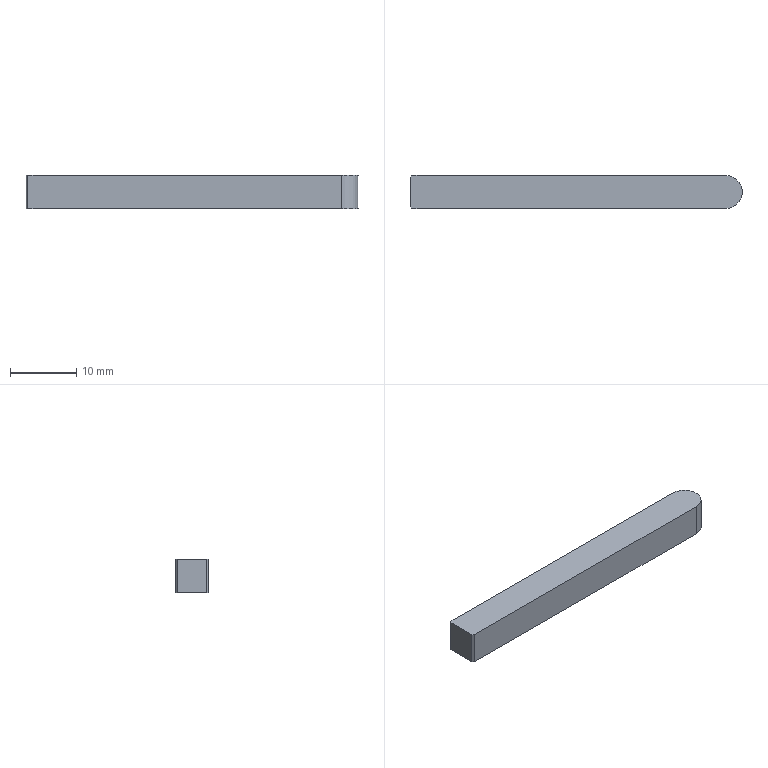Part | STEP file | BLC13-B5-L50^Magnetic powder brake assembly | 1 solid | 8 faces | box 50 x 5 x 5 mm | volume 1236 mm3 | plane 7 | cylinder 1 | commonest cylinder face diameters 5 x1
STEP:
#1=CARTESIAN_POINT('',(0.,0.,0.));
#2=DIRECTION('',(0.,0.,1.));
#3=DIRECTION('',(1.,0.,0.));
#4=AXIS2_PLACEMENT_3D('',#1,#2,#3);
#5=CARTESIAN_POINT('',(-25.,-2.2,0.));
#6=VERTEX_POINT('',#5);
#7=CARTESIAN_POINT('',(-24.7,-2.5,0.));
#8=VERTEX_POINT('',#7);
#9=CARTESIAN_POINT('',(-25.,-2.2,0.));
#10=DIRECTION('',(0.7071,-0.7071,0.));
#11=VECTOR('',#10,1.);
#12=LINE('',#9,#11);
#13=CARTESIAN_POINT('',(-25.,-2.2,5.));
#14=DIRECTION('',(0.7071,0.7071,0.));
#15=DIRECTION('',(0.,0.,-1.));
#16=AXIS2_PLACEMENT_3D('',#13,#14,#15);
#17=PLANE('',#16);
#18=CARTESIAN_POINT('',(5.,0.));
#19=DIRECTION('',(0.,-1.));
#20=VECTOR('',#19,1.);
#21=LINE('',#18,#20);
#22=(GEOMETRIC_REPRESENTATION_CONTEXT(2)PARAMETRIC_REPRESENTATION_CONTEXT()REPRESENTATION_CONTEXT('',''));
#23=DEFINITIONAL_REPRESENTATION('',(#21),#22);
#24=PCURVE('',#17,#23);
#25=CARTESIAN_POINT('',(22.5,0.,0.));
#26=DIRECTION('',(0.,0.,1.));
#27=DIRECTION('',(1.,0.,0.));
#28=AXIS2_PLACEMENT_3D('',#25,#26,#27);
#29=PLANE('',#28);
#30=CARTESIAN_POINT('',(-47.5,-2.2));
#31=DIRECTION('',(0.7071,-0.7071));
#32=VECTOR('',#31,1.);
#33=LINE('',#30,#32);
#34=(GEOMETRIC_REPRESENTATION_CONTEXT(2)PARAMETRIC_REPRESENTATION_CONTEXT()REPRESENTATION_CONTEXT('',''));
#35=DEFINITIONAL_REPRESENTATION('',(#33),#34);
#36=PCURVE('',#29,#35);
#37=SURFACE_CURVE('',#12,(#24,#36),.PCURVE_S1.);
#38=EDGE_CURVE('',#6,#8,#37,.T.);
#39=ORIENTED_EDGE('',*,*,#38,.T.);
#40=CARTESIAN_POINT('',(-24.7,-2.5,5.));
#41=VERTEX_POINT('',#40);
#42=CARTESIAN_POINT('',(-24.7,-2.5,5.));
#43=DIRECTION('',(0.,0.,-1.));
#44=VECTOR('',#43,1.);
#45=LINE('',#42,#44);
#46=CARTESIAN_POINT('',(0.,-0.4243));
#47=DIRECTION('',(1.,0.));
#48=VECTOR('',#47,1.);
#49=LINE('',#46,#48);
#50=(GEOMETRIC_REPRESENTATION_CONTEXT(2)PARAMETRIC_REPRESENTATION_CONTEXT()REPRESENTATION_CONTEXT('',''));
#51=DEFINITIONAL_REPRESENTATION('',(#49),#50);
#52=PCURVE('',#17,#51);
#53=CARTESIAN_POINT('',(-24.7,-2.5,5.));
#54=DIRECTION('',(0.,1.,0.));
#55=DIRECTION('',(1.,0.,0.));
#56=AXIS2_PLACEMENT_3D('',#53,#54,#55);
#57=PLANE('',#56);
#58=CARTESIAN_POINT('',(0.,0.));
#59=DIRECTION('',(0.,1.));
#60=VECTOR('',#59,1.);
#61=LINE('',#58,#60);
#62=(GEOMETRIC_REPRESENTATION_CONTEXT(2)PARAMETRIC_REPRESENTATION_CONTEXT()REPRESENTATION_CONTEXT('',''));
#63=DEFINITIONAL_REPRESENTATION('',(#61),#62);
#64=PCURVE('',#57,#63);
#65=SURFACE_CURVE('',#45,(#52,#64),.PCURVE_S1.);
#66=EDGE_CURVE('',#41,#8,#65,.T.);
#67=ORIENTED_EDGE('',*,*,#66,.F.);
#68=CARTESIAN_POINT('',(-25.,-2.2,5.));
#69=VERTEX_POINT('',#68);
#70=CARTESIAN_POINT('',(-25.,-2.2,5.));
#71=DIRECTION('',(0.7071,-0.7071,0.));
#72=VECTOR('',#71,1.);
#73=LINE('',#70,#72);
#74=CARTESIAN_POINT('',(0.,0.));
#75=DIRECTION('',(0.,-1.));
#76=VECTOR('',#75,1.);
#77=LINE('',#74,#76);
#78=(GEOMETRIC_REPRESENTATION_CONTEXT(2)PARAMETRIC_REPRESENTATION_CONTEXT()REPRESENTATION_CONTEXT('',''));
#79=DEFINITIONAL_REPRESENTATION('',(#77),#78);
#80=PCURVE('',#17,#79);
#81=CARTESIAN_POINT('',(22.5,0.,5.));
#82=DIRECTION('',(0.,0.,1.));
#83=DIRECTION('',(1.,0.,0.));
#84=AXIS2_PLACEMENT_3D('',#81,#82,#83);
#85=PLANE('',#84);
#86=CARTESIAN_POINT('',(-47.5,-2.2));
#87=DIRECTION('',(0.7071,-0.7071));
#88=VECTOR('',#87,1.);
#89=LINE('',#86,#88);
#90=(GEOMETRIC_REPRESENTATION_CONTEXT(2)PARAMETRIC_REPRESENTATION_CONTEXT()REPRESENTATION_CONTEXT('',''));
#91=DEFINITIONAL_REPRESENTATION('',(#89),#90);
#92=PCURVE('',#85,#91);
#93=SURFACE_CURVE('',#73,(#80,#92),.PCURVE_S1.);
#94=EDGE_CURVE('',#69,#41,#93,.T.);
#95=ORIENTED_EDGE('',*,*,#94,.F.);
#96=CARTESIAN_POINT('',(-25.,-2.2,5.));
#97=DIRECTION('',(0.,0.,-1.));
#98=VECTOR('',#97,1.);
#99=LINE('',#96,#98);
#100=CARTESIAN_POINT('',(0.,0.));
#101=DIRECTION('',(1.,0.));
#102=VECTOR('',#101,1.);
#103=LINE('',#100,#102);
#104=(GEOMETRIC_REPRESENTATION_CONTEXT(2)PARAMETRIC_REPRESENTATION_CONTEXT()REPRESENTATION_CONTEXT('',''));
#105=DEFINITIONAL_REPRESENTATION('',(#103),#104);
#106=PCURVE('',#17,#105);
#107=CARTESIAN_POINT('',(-25.,2.2,5.));
#108=DIRECTION('',(1.,0.,0.));
#109=DIRECTION('',(0.,1.,0.));
#110=AXIS2_PLACEMENT_3D('',#107,#108,#109);
#111=PLANE('',#110);
#112=CARTESIAN_POINT('',(-4.4,0.));
#113=DIRECTION('',(0.,-1.));
#114=VECTOR('',#113,1.);
#115=LINE('',#112,#114);
#116=(GEOMETRIC_REPRESENTATION_CONTEXT(2)PARAMETRIC_REPRESENTATION_CONTEXT()REPRESENTATION_CONTEXT('',''));
#117=DEFINITIONAL_REPRESENTATION('',(#115),#116);
#118=PCURVE('',#111,#117);
#119=SURFACE_CURVE('',#99,(#106,#118),.PCURVE_S1.);
#120=EDGE_CURVE('',#69,#6,#119,.T.);
#121=ORIENTED_EDGE('',*,*,#120,.T.);
#122=EDGE_LOOP('',(#39,#67,#95,#121));
#123=FACE_BOUND('',#122,.T.);
#124=ADVANCED_FACE('',(#123),#17,.F.);
#125=CARTESIAN_POINT('',(-24.7,2.5,0.));
#126=VERTEX_POINT('',#125);
#127=CARTESIAN_POINT('',(-25.,2.2,0.));
#128=VERTEX_POINT('',#127);
#129=CARTESIAN_POINT('',(-24.7,2.5,0.));
#130=DIRECTION('',(-0.7071,-0.7071,0.));
#131=VECTOR('',#130,1.);
#132=LINE('',#129,#131);
#133=CARTESIAN_POINT('',(-24.7,2.5,5.));
#134=DIRECTION('',(0.7071,-0.7071,0.));
#135=DIRECTION('',(0.,0.,-1.));
#136=AXIS2_PLACEMENT_3D('',#133,#134,#135);
#137=PLANE('',#136);
#138=CARTESIAN_POINT('',(5.,0.));
#139=DIRECTION('',(0.,-1.));
#140=VECTOR('',#139,1.);
#141=LINE('',#138,#140);
#142=(GEOMETRIC_REPRESENTATION_CONTEXT(2)PARAMETRIC_REPRESENTATION_CONTEXT()REPRESENTATION_CONTEXT('',''));
#143=DEFINITIONAL_REPRESENTATION('',(#141),#142);
#144=PCURVE('',#137,#143);
#145=CARTESIAN_POINT('',(-47.2,2.5));
#146=DIRECTION('',(-0.7071,-0.7071));
#147=VECTOR('',#146,1.);
#148=LINE('',#145,#147);
#149=(GEOMETRIC_REPRESENTATION_CONTEXT(2)PARAMETRIC_REPRESENTATION_CONTEXT()REPRESENTATION_CONTEXT('',''));
#150=DEFINITIONAL_REPRESENTATION('',(#148),#149);
#151=PCURVE('',#29,#150);
#152=SURFACE_CURVE('',#132,(#144,#151),.PCURVE_S1.);
#153=EDGE_CURVE('',#126,#128,#152,.T.);
#154=ORIENTED_EDGE('',*,*,#153,.T.);
#155=CARTESIAN_POINT('',(-25.,2.2,5.));
#156=VERTEX_POINT('',#155);
#157=CARTESIAN_POINT('',(-25.,2.2,5.));
#158=DIRECTION('',(0.,0.,-1.));
#159=VECTOR('',#158,1.);
#160=LINE('',#157,#159);
#161=CARTESIAN_POINT('',(0.,-0.4243));
#162=DIRECTION('',(1.,0.));
#163=VECTOR('',#162,1.);
#164=LINE('',#161,#163);
#165=(GEOMETRIC_REPRESENTATION_CONTEXT(2)PARAMETRIC_REPRESENTATION_CONTEXT()REPRESENTATION_CONTEXT('',''));
#166=DEFINITIONAL_REPRESENTATION('',(#164),#165);
#167=PCURVE('',#137,#166);
#168=CARTESIAN_POINT('',(0.,0.));
#169=DIRECTION('',(0.,-1.));
#170=VECTOR('',#169,1.);
#171=LINE('',#168,#170);
#172=(GEOMETRIC_REPRESENTATION_CONTEXT(2)PARAMETRIC_REPRESENTATION_CONTEXT()REPRESENTATION_CONTEXT('',''));
#173=DEFINITIONAL_REPRESENTATION('',(#171),#172);
#174=PCURVE('',#111,#173);
#175=SURFACE_CURVE('',#160,(#167,#174),.PCURVE_S1.);
#176=EDGE_CURVE('',#156,#128,#175,.T.);
#177=ORIENTED_EDGE('',*,*,#176,.F.);
#178=CARTESIAN_POINT('',(-24.7,2.5,5.));
#179=VERTEX_POINT('',#178);
#180=CARTESIAN_POINT('',(-24.7,2.5,5.));
#181=DIRECTION('',(-0.7071,-0.7071,0.));
#182=VECTOR('',#181,1.);
#183=LINE('',#180,#182);
#184=CARTESIAN_POINT('',(0.,0.));
#185=DIRECTION('',(0.,-1.));
#186=VECTOR('',#185,1.);
#187=LINE('',#184,#186);
#188=(GEOMETRIC_REPRESENTATION_CONTEXT(2)PARAMETRIC_REPRESENTATION_CONTEXT()REPRESENTATION_CONTEXT('',''));
#189=DEFINITIONAL_REPRESENTATION('',(#187),#188);
#190=PCURVE('',#137,#189);
#191=CARTESIAN_POINT('',(-47.2,2.5));
#192=DIRECTION('',(-0.7071,-0.7071));
#193=VECTOR('',#192,1.);
#194=LINE('',#191,#193);
#195=(GEOMETRIC_REPRESENTATION_CONTEXT(2)PARAMETRIC_REPRESENTATION_CONTEXT()REPRESENTATION_CONTEXT('',''));
#196=DEFINITIONAL_REPRESENTATION('',(#194),#195);
#197=PCURVE('',#85,#196);
#198=SURFACE_CURVE('',#183,(#190,#197),.PCURVE_S1.);
#199=EDGE_CURVE('',#179,#156,#198,.T.);
#200=ORIENTED_EDGE('',*,*,#199,.F.);
#201=CARTESIAN_POINT('',(-24.7,2.5,5.));
#202=DIRECTION('',(0.,0.,-1.));
#203=VECTOR('',#202,1.);
#204=LINE('',#201,#203);
#205=CARTESIAN_POINT('',(0.,0.));
#206=DIRECTION('',(1.,0.));
#207=VECTOR('',#206,1.);
#208=LINE('',#205,#207);
#209=(GEOMETRIC_REPRESENTATION_CONTEXT(2)PARAMETRIC_REPRESENTATION_CONTEXT()REPRESENTATION_CONTEXT('',''));
#210=DEFINITIONAL_REPRESENTATION('',(#208),#209);
#211=PCURVE('',#137,#210);
#212=CARTESIAN_POINT('',(22.5,2.5,5.));
#213=DIRECTION('',(0.,-1.,0.));
#214=DIRECTION('',(0.,0.,-1.));
#215=AXIS2_PLACEMENT_3D('',#212,#213,#214);
#216=PLANE('',#215);
#217=CARTESIAN_POINT('',(0.,-47.2));
#218=DIRECTION('',(1.,0.));
#219=VECTOR('',#218,1.);
#220=LINE('',#217,#219);
#221=(GEOMETRIC_REPRESENTATION_CONTEXT(2)PARAMETRIC_REPRESENTATION_CONTEXT()REPRESENTATION_CONTEXT('',''));
#222=DEFINITIONAL_REPRESENTATION('',(#220),#221);
#223=PCURVE('',#216,#222);
#224=SURFACE_CURVE('',#204,(#211,#223),.PCURVE_S1.);
#225=EDGE_CURVE('',#179,#126,#224,.T.);
#226=ORIENTED_EDGE('',*,*,#225,.T.);
#227=EDGE_LOOP('',(#154,#177,#200,#226));
#228=FACE_BOUND('',#227,.T.);
#229=ADVANCED_FACE('',(#228),#137,.F.);
#230=CARTESIAN_POINT('',(-25.,2.2,0.));
#231=DIRECTION('',(0.,-1.,0.));
#232=VECTOR('',#231,1.);
#233=LINE('',#230,#232);
#234=CARTESIAN_POINT('',(-47.5,2.2));
#235=DIRECTION('',(0.,-1.));
#236=VECTOR('',#235,1.);
#237=LINE('',#234,#236);
#238=(GEOMETRIC_REPRESENTATION_CONTEXT(2)PARAMETRIC_REPRESENTATION_CONTEXT()REPRESENTATION_CONTEXT('',''));
#239=DEFINITIONAL_REPRESENTATION('',(#237),#238);
#240=PCURVE('',#29,#239);
#241=CARTESIAN_POINT('',(0.,-5.));
#242=DIRECTION('',(-1.,0.));
#243=VECTOR('',#242,1.);
#244=LINE('',#241,#243);
#245=(GEOMETRIC_REPRESENTATION_CONTEXT(2)PARAMETRIC_REPRESENTATION_CONTEXT()REPRESENTATION_CONTEXT('',''));
#246=DEFINITIONAL_REPRESENTATION('',(#244),#245);
#247=PCURVE('',#111,#246);
#248=SURFACE_CURVE('',#233,(#240,#247),.PCURVE_S1.);
#249=EDGE_CURVE('',#128,#6,#248,.T.);
#250=ORIENTED_EDGE('',*,*,#249,.F.);
#251=ORIENTED_EDGE('',*,*,#153,.F.);
#252=CARTESIAN_POINT('',(22.5,2.5,0.));
#253=VERTEX_POINT('',#252);
#254=CARTESIAN_POINT('',(22.5,2.5,0.));
#255=DIRECTION('',(-1.,0.,0.));
#256=VECTOR('',#255,1.);
#257=LINE('',#254,#256);
#258=CARTESIAN_POINT('',(0.,2.5));
#259=DIRECTION('',(-1.,0.));
#260=VECTOR('',#259,1.);
#261=LINE('',#258,#260);
#262=(GEOMETRIC_REPRESENTATION_CONTEXT(2)PARAMETRIC_REPRESENTATION_CONTEXT()REPRESENTATION_CONTEXT('',''));
#263=DEFINITIONAL_REPRESENTATION('',(#261),#262);
#264=PCURVE('',#29,#263);
#265=CARTESIAN_POINT('',(5.,0.));
#266=DIRECTION('',(0.,-1.));
#267=VECTOR('',#266,1.);
#268=LINE('',#265,#267);
#269=(GEOMETRIC_REPRESENTATION_CONTEXT(2)PARAMETRIC_REPRESENTATION_CONTEXT()REPRESENTATION_CONTEXT('',''));
#270=DEFINITIONAL_REPRESENTATION('',(#268),#269);
#271=PCURVE('',#216,#270);
#272=SURFACE_CURVE('',#257,(#264,#271),.PCURVE_S1.);
#273=EDGE_CURVE('',#253,#126,#272,.T.);
#274=ORIENTED_EDGE('',*,*,#273,.F.);
#275=CARTESIAN_POINT('',(22.5,-2.5,0.));
#276=VERTEX_POINT('',#275);
#277=CARTESIAN_POINT('',(22.5,0.,0.));
#278=DIRECTION('',(0.,0.,1.));
#279=DIRECTION('',(1.,0.,0.));
#280=AXIS2_PLACEMENT_3D('',#277,#278,#279);
#281=CIRCLE('',#280,2.5);
#282=CARTESIAN_POINT('',(0.,0.));
#283=DIRECTION('',(1.,0.));
#284=AXIS2_PLACEMENT_2D('',#282,#283);
#285=CIRCLE('',#284,2.5);
#286=(GEOMETRIC_REPRESENTATION_CONTEXT(2)PARAMETRIC_REPRESENTATION_CONTEXT()REPRESENTATION_CONTEXT('',''));
#287=DEFINITIONAL_REPRESENTATION('',(#285),#286);
#288=PCURVE('',#29,#287);
#289=CARTESIAN_POINT('',(22.5,0.,5.));
#290=DIRECTION('',(0.,0.,1.));
#291=DIRECTION('',(-1.,0.,0.));
#292=AXIS2_PLACEMENT_3D('',#289,#290,#291);
#293=CYLINDRICAL_SURFACE('',#292,2.5);
#294=CARTESIAN_POINT('',(-3.142,-5.));
#295=DIRECTION('',(1.,0.));
#296=VECTOR('',#295,1.);
#297=LINE('',#294,#296);
#298=(GEOMETRIC_REPRESENTATION_CONTEXT(2)PARAMETRIC_REPRESENTATION_CONTEXT()REPRESENTATION_CONTEXT('',''));
#299=DEFINITIONAL_REPRESENTATION('',(#297),#298);
#300=PCURVE('',#293,#299);
#301=SURFACE_CURVE('',#281,(#288,#300),.PCURVE_S1.);
#302=EDGE_CURVE('',#276,#253,#301,.T.);
#303=ORIENTED_EDGE('',*,*,#302,.F.);
#304=CARTESIAN_POINT('',(-24.7,-2.5,0.));
#305=DIRECTION('',(1.,0.,0.));
#306=VECTOR('',#305,1.);
#307=LINE('',#304,#306);
#308=CARTESIAN_POINT('',(-47.2,-2.5));
#309=DIRECTION('',(1.,0.));
#310=VECTOR('',#309,1.);
#311=LINE('',#308,#310);
#312=(GEOMETRIC_REPRESENTATION_CONTEXT(2)PARAMETRIC_REPRESENTATION_CONTEXT()REPRESENTATION_CONTEXT('',''));
#313=DEFINITIONAL_REPRESENTATION('',(#311),#312);
#314=PCURVE('',#29,#313);
#315=CARTESIAN_POINT('',(0.,5.));
#316=DIRECTION('',(1.,0.));
#317=VECTOR('',#316,1.);
#318=LINE('',#315,#317);
#319=(GEOMETRIC_REPRESENTATION_CONTEXT(2)PARAMETRIC_REPRESENTATION_CONTEXT()REPRESENTATION_CONTEXT('',''));
#320=DEFINITIONAL_REPRESENTATION('',(#318),#319);
#321=PCURVE('',#57,#320);
#322=SURFACE_CURVE('',#307,(#314,#321),.PCURVE_S1.);
#323=EDGE_CURVE('',#8,#276,#322,.T.);
#324=ORIENTED_EDGE('',*,*,#323,.F.);
#325=ORIENTED_EDGE('',*,*,#38,.F.);
#326=EDGE_LOOP('',(#250,#251,#274,#303,#324,#325));
#327=FACE_BOUND('',#326,.T.);
#328=ADVANCED_FACE('',(#327),#29,.F.);
#329=ORIENTED_EDGE('',*,*,#323,.T.);
#330=CARTESIAN_POINT('',(22.5,-2.5,5.));
#331=VERTEX_POINT('',#330);
#332=CARTESIAN_POINT('',(22.5,-2.5,5.));
#333=DIRECTION('',(0.,0.,-1.));
#334=VECTOR('',#333,1.);
#335=LINE('',#332,#334);
#336=CARTESIAN_POINT('',(47.2,0.));
#337=DIRECTION('',(0.,1.));
#338=VECTOR('',#337,1.);
#339=LINE('',#336,#338);
#340=(GEOMETRIC_REPRESENTATION_CONTEXT(2)PARAMETRIC_REPRESENTATION_CONTEXT()REPRESENTATION_CONTEXT('',''));
#341=DEFINITIONAL_REPRESENTATION('',(#339),#340);
#342=PCURVE('',#57,#341);
#343=CARTESIAN_POINT('',(1.571,0.));
#344=DIRECTION('',(0.,-1.));
#345=VECTOR('',#344,1.);
#346=LINE('',#343,#345);
#347=(GEOMETRIC_REPRESENTATION_CONTEXT(2)PARAMETRIC_REPRESENTATION_CONTEXT()REPRESENTATION_CONTEXT('',''));
#348=DEFINITIONAL_REPRESENTATION('',(#346),#347);
#349=PCURVE('',#293,#348);
#350=SURFACE_CURVE('',#335,(#342,#349),.PCURVE_S1.);
#351=EDGE_CURVE('',#331,#276,#350,.T.);
#352=ORIENTED_EDGE('',*,*,#351,.F.);
#353=CARTESIAN_POINT('',(-24.7,-2.5,5.));
#354=DIRECTION('',(1.,0.,0.));
#355=VECTOR('',#354,1.);
#356=LINE('',#353,#355);
#357=CARTESIAN_POINT('',(0.,0.));
#358=DIRECTION('',(1.,0.));
#359=VECTOR('',#358,1.);
#360=LINE('',#357,#359);
#361=(GEOMETRIC_REPRESENTATION_CONTEXT(2)PARAMETRIC_REPRESENTATION_CONTEXT()REPRESENTATION_CONTEXT('',''));
#362=DEFINITIONAL_REPRESENTATION('',(#360),#361);
#363=PCURVE('',#57,#362);
#364=CARTESIAN_POINT('',(-47.2,-2.5));
#365=DIRECTION('',(1.,0.));
#366=VECTOR('',#365,1.);
#367=LINE('',#364,#366);
#368=(GEOMETRIC_REPRESENTATION_CONTEXT(2)PARAMETRIC_REPRESENTATION_CONTEXT()REPRESENTATION_CONTEXT('',''));
#369=DEFINITIONAL_REPRESENTATION('',(#367),#368);
#370=PCURVE('',#85,#369);
#371=SURFACE_CURVE('',#356,(#363,#370),.PCURVE_S1.);
#372=EDGE_CURVE('',#41,#331,#371,.T.);
#373=ORIENTED_EDGE('',*,*,#372,.F.);
#374=ORIENTED_EDGE('',*,*,#66,.T.);
#375=EDGE_LOOP('',(#329,#352,#373,#374));
#376=FACE_BOUND('',#375,.T.);
#377=ADVANCED_FACE('',(#376),#57,.F.);
#378=ORIENTED_EDGE('',*,*,#273,.T.);
#379=ORIENTED_EDGE('',*,*,#225,.F.);
#380=CARTESIAN_POINT('',(22.5,2.5,5.));
#381=VERTEX_POINT('',#380);
#382=CARTESIAN_POINT('',(22.5,2.5,5.));
#383=DIRECTION('',(-1.,0.,0.));
#384=VECTOR('',#383,1.);
#385=LINE('',#382,#384);
#386=CARTESIAN_POINT('',(0.,0.));
#387=DIRECTION('',(0.,-1.));
#388=VECTOR('',#387,1.);
#389=LINE('',#386,#388);
#390=(GEOMETRIC_REPRESENTATION_CONTEXT(2)PARAMETRIC_REPRESENTATION_CONTEXT()REPRESENTATION_CONTEXT('',''));
#391=DEFINITIONAL_REPRESENTATION('',(#389),#390);
#392=PCURVE('',#216,#391);
#393=CARTESIAN_POINT('',(0.,2.5));
#394=DIRECTION('',(-1.,0.));
#395=VECTOR('',#394,1.);
#396=LINE('',#393,#395);
#397=(GEOMETRIC_REPRESENTATION_CONTEXT(2)PARAMETRIC_REPRESENTATION_CONTEXT()REPRESENTATION_CONTEXT('',''));
#398=DEFINITIONAL_REPRESENTATION('',(#396),#397);
#399=PCURVE('',#85,#398);
#400=SURFACE_CURVE('',#385,(#392,#399),.PCURVE_S1.);
#401=EDGE_CURVE('',#381,#179,#400,.T.);
#402=ORIENTED_EDGE('',*,*,#401,.F.);
#403=CARTESIAN_POINT('',(22.5,2.5,5.));
#404=DIRECTION('',(0.,0.,-1.));
#405=VECTOR('',#404,1.);
#406=LINE('',#403,#405);
#407=CARTESIAN_POINT('',(0.,0.));
#408=DIRECTION('',(1.,0.));
#409=VECTOR('',#408,1.);
#410=LINE('',#407,#409);
#411=(GEOMETRIC_REPRESENTATION_CONTEXT(2)PARAMETRIC_REPRESENTATION_CONTEXT()REPRESENTATION_CONTEXT('',''));
#412=DEFINITIONAL_REPRESENTATION('',(#410),#411);
#413=PCURVE('',#216,#412);
#414=CARTESIAN_POINT('',(4.712,0.));
#415=DIRECTION('',(0.,-1.));
#416=VECTOR('',#415,1.);
#417=LINE('',#414,#416);
#418=(GEOMETRIC_REPRESENTATION_CONTEXT(2)PARAMETRIC_REPRESENTATION_CONTEXT()REPRESENTATION_CONTEXT('',''));
#419=DEFINITIONAL_REPRESENTATION('',(#417),#418);
#420=PCURVE('',#293,#419);
#421=SURFACE_CURVE('',#406,(#413,#420),.PCURVE_S1.);
#422=EDGE_CURVE('',#381,#253,#421,.T.);
#423=ORIENTED_EDGE('',*,*,#422,.T.);
#424=EDGE_LOOP('',(#378,#379,#402,#423));
#425=FACE_BOUND('',#424,.T.);
#426=ADVANCED_FACE('',(#425),#216,.F.);
#427=ORIENTED_EDGE('',*,*,#302,.T.);
#428=ORIENTED_EDGE('',*,*,#422,.F.);
#429=CARTESIAN_POINT('',(22.5,0.,5.));
#430=DIRECTION('',(0.,0.,1.));
#431=DIRECTION('',(1.,0.,0.));
#432=AXIS2_PLACEMENT_3D('',#429,#430,#431);
#433=CIRCLE('',#432,2.5);
#434=CARTESIAN_POINT('',(-3.142,0.));
#435=DIRECTION('',(1.,0.));
#436=VECTOR('',#435,1.);
#437=LINE('',#434,#436);
#438=(GEOMETRIC_REPRESENTATION_CONTEXT(2)PARAMETRIC_REPRESENTATION_CONTEXT()REPRESENTATION_CONTEXT('',''));
#439=DEFINITIONAL_REPRESENTATION('',(#437),#438);
#440=PCURVE('',#293,#439);
#441=CARTESIAN_POINT('',(0.,0.));
#442=DIRECTION('',(1.,0.));
#443=AXIS2_PLACEMENT_2D('',#441,#442);
#444=CIRCLE('',#443,2.5);
#445=(GEOMETRIC_REPRESENTATION_CONTEXT(2)PARAMETRIC_REPRESENTATION_CONTEXT()REPRESENTATION_CONTEXT('',''));
#446=DEFINITIONAL_REPRESENTATION('',(#444),#445);
#447=PCURVE('',#85,#446);
#448=SURFACE_CURVE('',#433,(#440,#447),.PCURVE_S1.);
#449=EDGE_CURVE('',#331,#381,#448,.T.);
#450=ORIENTED_EDGE('',*,*,#449,.F.);
#451=ORIENTED_EDGE('',*,*,#351,.T.);
#452=EDGE_LOOP('',(#427,#428,#450,#451));
#453=FACE_BOUND('',#452,.T.);
#454=ADVANCED_FACE('',(#453),#293,.T.);
#455=CARTESIAN_POINT('',(-25.,2.2,5.));
#456=DIRECTION('',(0.,-1.,0.));
#457=VECTOR('',#456,1.);
#458=LINE('',#455,#457);
#459=CARTESIAN_POINT('',(-47.5,2.2));
#460=DIRECTION('',(0.,-1.));
#461=VECTOR('',#460,1.);
#462=LINE('',#459,#461);
#463=(GEOMETRIC_REPRESENTATION_CONTEXT(2)PARAMETRIC_REPRESENTATION_CONTEXT()REPRESENTATION_CONTEXT('',''));
#464=DEFINITIONAL_REPRESENTATION('',(#462),#463);
#465=PCURVE('',#85,#464);
#466=CARTESIAN_POINT('',(0.,0.));
#467=DIRECTION('',(-1.,0.));
#468=VECTOR('',#467,1.);
#469=LINE('',#466,#468);
#470=(GEOMETRIC_REPRESENTATION_CONTEXT(2)PARAMETRIC_REPRESENTATION_CONTEXT()REPRESENTATION_CONTEXT('',''));
#471=DEFINITIONAL_REPRESENTATION('',(#469),#470);
#472=PCURVE('',#111,#471);
#473=SURFACE_CURVE('',#458,(#465,#472),.PCURVE_S1.);
#474=EDGE_CURVE('',#156,#69,#473,.T.);
#475=ORIENTED_EDGE('',*,*,#474,.T.);
#476=ORIENTED_EDGE('',*,*,#94,.T.);
#477=ORIENTED_EDGE('',*,*,#372,.T.);
#478=ORIENTED_EDGE('',*,*,#449,.T.);
#479=ORIENTED_EDGE('',*,*,#401,.T.);
#480=ORIENTED_EDGE('',*,*,#199,.T.);
#481=EDGE_LOOP('',(#475,#476,#477,#478,#479,#480));
#482=FACE_BOUND('',#481,.T.);
#483=ADVANCED_FACE('',(#482),#85,.T.);
#484=ORIENTED_EDGE('',*,*,#249,.T.);
#485=ORIENTED_EDGE('',*,*,#120,.F.);
#486=ORIENTED_EDGE('',*,*,#474,.F.);
#487=ORIENTED_EDGE('',*,*,#176,.T.);
#488=EDGE_LOOP('',(#484,#485,#486,#487));
#489=FACE_BOUND('',#488,.T.);
#490=ADVANCED_FACE('',(#489),#111,.F.);
#491=CLOSED_SHELL('',(#124,#229,#328,#377,#426,#454,#483,#490));
#492=MANIFOLD_SOLID_BREP('',#491);
#493=(LENGTH_UNIT()NAMED_UNIT(*)SI_UNIT(.MILLI.,.METRE.));
#494=UNCERTAINTY_MEASURE_WITH_UNIT(LENGTH_MEASURE(0.0000001),#493,'','');
#495=(NAMED_UNIT(*)PLANE_ANGLE_UNIT()SI_UNIT($,.RADIAN.));
#496=(NAMED_UNIT(*)SI_UNIT($,.STERADIAN.)SOLID_ANGLE_UNIT());
#497=(GEOMETRIC_REPRESENTATION_CONTEXT(3)GLOBAL_UNCERTAINTY_ASSIGNED_CONTEXT((#494))GLOBAL_UNIT_ASSIGNED_CONTEXT((#493,#495,#496))REPRESENTATION_CONTEXT('',''));
#498=ADVANCED_BREP_SHAPE_REPRESENTATION('',(#4,#492),#497);